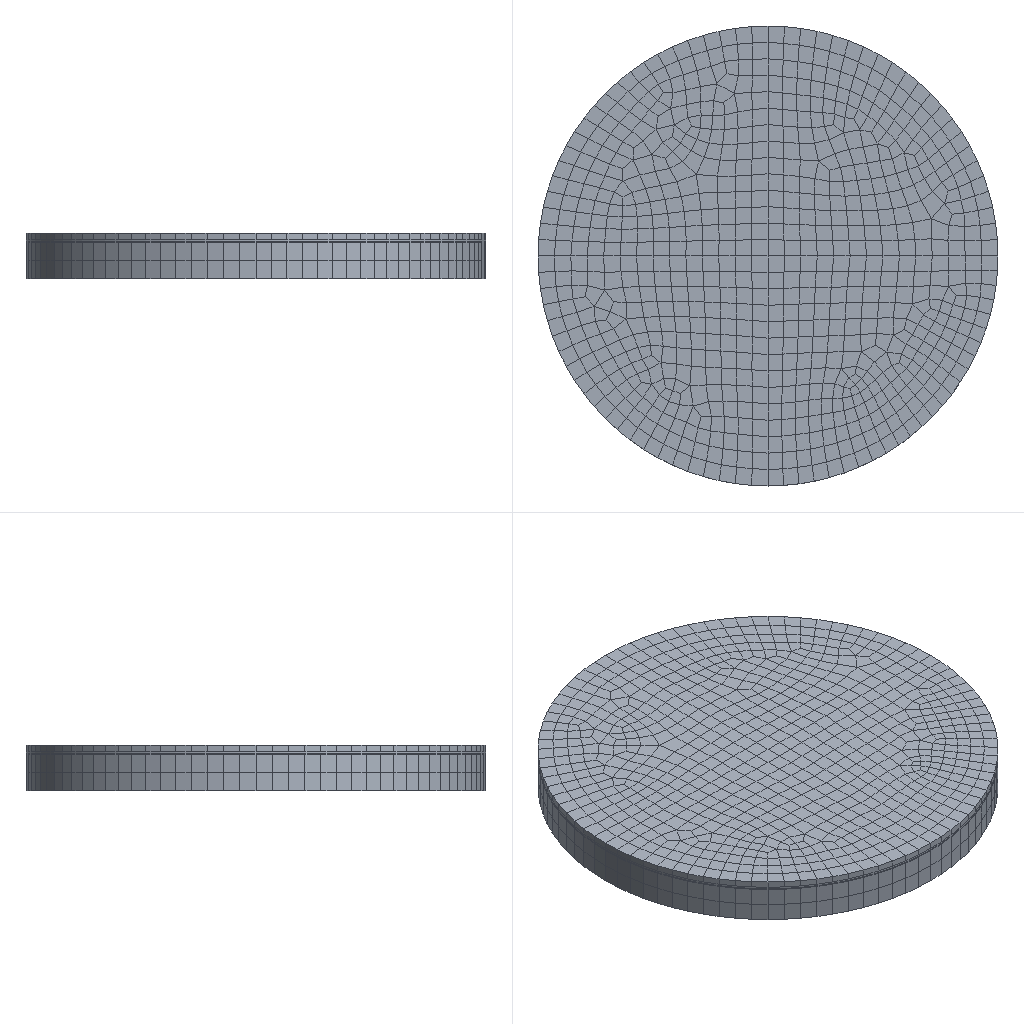Simulation study | abaqus
Set-up summary:
category,name,step,type,value,unit,region
solver,abaqus
solver,version,,,Abaqus/Standard 2020
units,not stated in the deck,,not stated
analysis,deck,,coupled temperature-displacement,coupled temperature-displacement
load_step,Step-1,Step-1,coupled temperature-displacement
load_step,requested,,,1
mesh,nodes,,,4866
mesh,elements,,,3825
element_type,C3D8RT,,solid,3825
load,load commands in deck,,count,3
bc,support commands in deck,,count,1
material,JIDI,,in results
material,RUAN,,in results
material,YING,,in results
material,ZHONG,,in results
check,setup vs results,,match,"per instance, exact: element labels, types and connectivity; labels of the nodes the elements use; coordinates of those nodes at SINGLE_PRECISION in 1 of 1 instance(s)"
Abaqus input file, long lists of numbers shortened:
*Heading
** Job name: Job-1 Model name: Model-1
** Generated by: Abaqus/CAE 2020
*Preprint, echo=NO, model=NO, history=NO, contact=NO
**
** PARTS
**
*Part, name=Part-1
*Node
      1,           0.,           0., 0.00172
      2, -0.01,           0., 0.00172
** (4864 more lines like these left out)
*Element, type=C3D8RT
  1,  860,  868,  866,  861, 1021, 1029, 1027, 1022
  2,  855,  850,  828,  831, 1016, 1011,  989,  992
** (3823 more lines like these left out)
*Nset, nset=Set-10
   10,   11,   12,   13,   14,   15,   16,   24,   25,   26,   27,   28,  172,  173,  174,  175
  176,  177,  178,  179,  180,  181,  182,  183,  184,  185,  186,  187,  188,  189,  190,  191
** (151 more lines like these left out)
*Elset, elset=Set-10
  556,  557,  558,  559,  560,  561,  562,  563,  564,  565,  566,  567,  568,  569,  570,  571
  572,  573,  574,  575,  576,  577,  578,  579,  580,  581,  582,  583,  584,  585,  586,  587
** (94 more lines like these left out)
*Nset, nset=Set-11
    7,    8,    9,   10,   11,   12,   16,   17,   22,   23,   24,   25,  125,  126,  127,  128
  129,  130,  131,  132,  133,  134,  135,  136,  137,  138,  139,  140,  141,  142,  143,  144
** (100 more lines like these left out)
*Elset, elset=Set-11
  371,  372,  373,  374,  375,  376,  377,  378,  379,  380,  381,  382,  383,  384,  385,  386
  387,  388,  389,  390,  391,  392,  393,  394,  395,  396,  397,  398,  399,  400,  401,  402
** (46 more lines like these left out)
*Nset, nset=Set-12
    1,    2,    3,    7,    8,    9,   17,   18,   20,   21,   22,   23,   31,   32,   33,   34
   35,   36,   37,   38,   39,   40,   41,   42,   43,   44,   45,   46,   47,   48,   49,   50
** (100 more lines like these left out)
*Elset, elset=Set-12
  186,  187,  188,  189,  190,  191,  192,  193,  194,  195,  196,  197,  198,  199,  200,  201
  202,  203,  204,  205,  206,  207,  208,  209,  210,  211,  212,  213,  214,  215,  216,  217
** (46 more lines like these left out)
*Nset, nset=Set-13
    1,    2,    3,    4,    5,    6,   18,   19,   20,   21,   29,   30,   31,   32,   33,   34
   35,   36,   37,   38,   39,   40,   41,   42,   43,   44,   45,   46,   47,   48,   49,   50
** (100 more lines like these left out)
*Elset, elset=Set-13
    1,    2,    3,    4,    5,    6,    7,    8,    9,   10,   11,   12,   13,   14,   15,   16
   17,   18,   19,   20,   21,   22,   23,   24,   25,   26,   27,   28,   29,   30,   31,   32
** (46 more lines like these left out)
** Section: ying
*Solid Section, elset=Set-13, material=ying
,
** Section: zhong
*Solid Section, elset=Set-12, material=zhong
,
** Section: ruan
*Solid Section, elset=Set-11, material=ruan
,
** Section: jidi
*Solid Section, elset=Set-10, material=jidi
,
*End Part
**
**
** ASSEMBLY
**
*Assembly, name=Assembly
**
*Instance, name=Part-1-1, part=Part-1
*End Instance
**
*Nset, nset=Set-1, instance=Part-1-1
 27, 30
*Nset, nset=Set-2, instance=Part-1-1
 27, 30
*Nset, nset=Set-3, instance=Part-1-1, generate
    1,  4866,     1
*Elset, elset=Set-3, instance=Part-1-1, generate
    1,  3825,     1
*Nset, nset=Set-4, instance=Part-1-1, generate
    1,  4866,     1
*Elset, elset=Set-4, instance=Part-1-1, generate
    1,  3825,     1
*Elset, elset=_Surf-3_S2, internal, instance=Part-1-1
    1,    2,    3,    4,    5,    6,    7,    8,    9,   10,   11,   12,   13,   14,   15,   16
   17,   18,   19,   20,   21,   22,   23,   24,   25,   26,   27,   28,   29,   30,   31,   32
** (94 more lines like these left out)
*Elset, elset=_Surf-3_S4, internal, instance=Part-1-1
   10,   11,   17,   19,   22,   25,   27,   30,   46,   48,   51,   54,   56,   58,   99, 2322
 2326, 2338, 2339, 2346, 2348, 2370, 2371, 2374, 2375, 2379, 2393, 2525, 2526, 2530, 2539, 2542
** (3 more lines like these left out)
*Elset, elset=_Surf-3_S6, internal, instance=Part-1-1
    4,    8,   14,   21,   23,   31,   32, 2323, 2329, 2330, 2331, 2332, 2334, 2337, 2340, 2343
 2347, 2364, 2365, 2524, 2531, 2536, 2555, 2556, 2561, 2566, 2572, 2574, 3454, 3466, 3475, 3478
** (1 more lines like these left out)
*Elset, elset=_Surf-3_S3, internal, instance=Part-1-1
  189,  193,  199,  206,  208,  216,  217,  374,  378,  384,  391,  393,  401,  402,  559,  563
  569,  576,  578,  586,  587,  744,  748,  754,  761,  763,  771,  772,  926,  938,  947,  950
** (7 more lines like these left out)
*Elset, elset=_Surf-3_S5, internal, instance=Part-1-1
  195,  196,  202,  204,  207,  210,  212,  215,  231,  233,  236,  239,  241,  243,  284,  380
  381,  387,  389,  392,  395,  397,  400,  416,  418,  421,  424,  426,  428,  469,  565,  566
** (11 more lines like these left out)
*Surface, type=ELEMENT, name=Surf-3
_Surf-3_S2, S2
_Surf-3_S4, S4
_Surf-3_S6, S6
_Surf-3_S3, S3
_Surf-3_S5, S5
*Elset, elset=_Surf-4_S2, internal, instance=Part-1-1
    1,    2,    3,    4,    5,    6,    7,    8,    9,   10,   11,   12,   13,   14,   15,   16
   17,   18,   19,   20,   21,   22,   23,   24,   25,   26,   27,   28,   29,   30,   31,   32
** (94 more lines like these left out)
*Elset, elset=_Surf-4_S4, internal, instance=Part-1-1
   10,   11,   17,   19,   22,   25,   27,   30,   46,   48,   51,   54,   56,   58,   99, 2322
 2326, 2338, 2339, 2346, 2348, 2370, 2371, 2374, 2375, 2379, 2393, 2525, 2526, 2530, 2539, 2542
** (3 more lines like these left out)
*Elset, elset=_Surf-4_S6, internal, instance=Part-1-1
    4,    8,   14,   21,   23,   31,   32, 2323, 2329, 2330, 2331, 2332, 2334, 2337, 2340, 2343
 2347, 2364, 2365, 2524, 2531, 2536, 2555, 2556, 2561, 2566, 2572, 2574, 3454, 3466, 3475, 3478
** (1 more lines like these left out)
*Elset, elset=_Surf-4_S3, internal, instance=Part-1-1
  189,  193,  199,  206,  208,  216,  217,  374,  378,  384,  391,  393,  401,  402,  559,  563
  569,  576,  578,  586,  587,  744,  748,  754,  761,  763,  771,  772,  926,  938,  947,  950
** (7 more lines like these left out)
*Elset, elset=_Surf-4_S5, internal, instance=Part-1-1
  195,  196,  202,  204,  207,  210,  212,  215,  231,  233,  236,  239,  241,  243,  284,  380
  381,  387,  389,  392,  395,  397,  400,  416,  418,  421,  424,  426,  428,  469,  565,  566
** (11 more lines like these left out)
*Surface, type=ELEMENT, name=Surf-4
_Surf-4_S2, S2
_Surf-4_S4, S4
_Surf-4_S6, S6
_Surf-4_S3, S3
_Surf-4_S5, S5
*End Assembly
*Amplitude, name=Amp-1
             0.,              0.,             50.,              1.
**
** MATERIALS
**
*Material, name=jidi
*Conductivity
42.,
*Density
 1.54e-09,
*Elastic
630000., 0.26
*Expansion
 4.9e-06,
*Specific Heat
 4.2e+08,
*Material, name=ruan
*Conductivity
 0.15,
*Density
 3.4e-09,
*Elastic
625000., 0.3
*Expansion
 6.2e-06,
*Specific Heat
 6.2e+08,
*Material, name=ying
*Conductivity
 0.15,
*Density
 3.4e-09,
*Elastic
685000., 0.3
*Expansion
 6.2e-06,
*Specific Heat
 1.5e+08,
*Material, name=zhong
*Conductivity
 0.15,
*Density
 3.4e-09,
*Elastic
645000., 0.3
*Expansion
 6.2e-06,
*Specific Heat
 6.22e+08,
**
** PHYSICAL CONSTANTS
**
*Physical Constants, absolute zero=-273., stefan boltzmann=5.67e-08
**
** PREDEFINED FIELDS
**
** Name: Predefined Field-1   Type: Temperature
*Initial Conditions, type=TEMPERATURE
Set-4, 20.
** ----------------------------------------------------------------
**
** STEP: Step-1
**
*Step, name=Step-1, nlgeom=YES, inc=1000
*Coupled Temperature-displacement, creep=none, steady state, stabilize=0.0002, allsdtol=0.05, continue=NO
0.01, 50., 1e-05, 50.
**
** BOUNDARY CONDITIONS
**
** Name: BC-1 Type: 温度
*Boundary, amplitude=Amp-1
Set-3, 11, 11, 670.
**
** INTERACTIONS
**
** Interaction: Int-1
*Sfilm
Surf-3, F, 20., 0.001
** Interaction: Int-2
*Sradiate
Surf-4, R, 20., 0.5
**
** OUTPUT REQUESTS
**
*Restart, write, frequency=0
**
** FIELD OUTPUT: F-Output-1
**
*Output, field
*Node Output
CF, NT, RF, RFL, U, V
*Element Output, directions=YES
E, HFL, LE, MISES, PE, PEEQ, PEMAG, S, TEMP
*Contact Output
CDISP, CSTRESS
**
** HISTORY OUTPUT: H-Output-1
**
*Output, history, variable=PRESELECT
*End Step
Results summary:
result,step,,completed,increments=21 time=50.0/50.0
result,analysis,,,"coupled temperature-displacement, steady state"
result,last_loadstep,,,1
result,primary field,,,"U, NT11"
result,reaction total,,FX,0.0,model units
result,reaction total,,FY,0.0,model units
result,reaction total,,FZ,0.0,model units